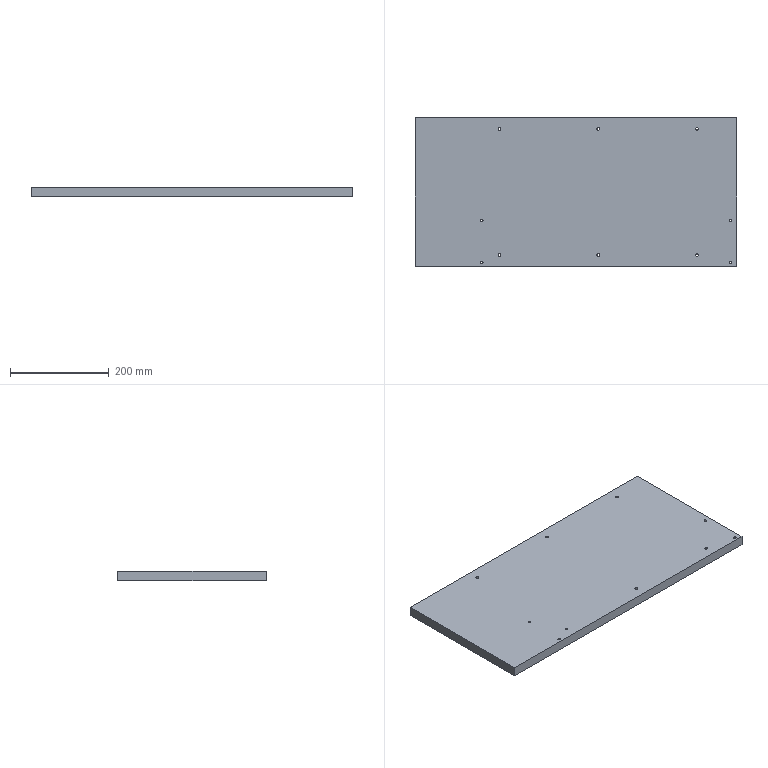Part | SolidWorks | features BaseBody 1 | 1 solid | 44 faces | box 650 x 300 x 20 mm | volume 3893705 mm3 | cylinder 32 | plane 12 | commonest cylinder face diameters 5.5 x12 10 x12 5 x8
STEP:
#1=CARTESIAN_POINT('',(240.,-127.5,5.7));
#2=VERTEX_POINT('',#1);
#3=CARTESIAN_POINT('',(250.,-127.5,5.7));
#4=VERTEX_POINT('',#3);
#5=CARTESIAN_POINT('',(245.,-127.5,5.7));
#6=DIRECTION('',(0.,0.,1.));
#7=DIRECTION('',(-1.,0.,0.));
#8=AXIS2_PLACEMENT_3D('',#5,#6,#7);
#9=CIRCLE('',#8,5.);
#10=EDGE_CURVE('',#2,#4,#9,.T.);
#11=ORIENTED_EDGE('',*,*,#10,.T.);
#12=CARTESIAN_POINT('',(250.,-127.5,0.));
#13=VERTEX_POINT('',#12);
#14=CARTESIAN_POINT('',(250.,-127.5,5.7));
#15=DIRECTION('',(0.,0.,-1.));
#16=VECTOR('',#15,1000.);
#17=LINE('',#14,#16);
#18=EDGE_CURVE('',#4,#13,#17,.T.);
#19=ORIENTED_EDGE('',*,*,#18,.T.);
#20=CARTESIAN_POINT('',(240.,-127.5,0.));
#21=VERTEX_POINT('',#20);
#22=CARTESIAN_POINT('',(245.,-127.5,0.));
#23=DIRECTION('',(0.,0.,-1.));
#24=DIRECTION('',(-1.,0.,0.));
#25=AXIS2_PLACEMENT_3D('',#22,#23,#24);
#26=CIRCLE('',#25,5.);
#27=EDGE_CURVE('',#13,#21,#26,.T.);
#28=ORIENTED_EDGE('',*,*,#27,.T.);
#29=CARTESIAN_POINT('',(240.,-127.5,5.7));
#30=DIRECTION('',(0.,0.,-1.));
#31=VECTOR('',#30,1000.);
#32=LINE('',#29,#31);
#33=EDGE_CURVE('',#2,#21,#32,.T.);
#34=ORIENTED_EDGE('',*,*,#33,.F.);
#35=EDGE_LOOP('',(#11,#19,#28,#34));
#36=FACE_OUTER_BOUND('',#35,.T.);
#37=CARTESIAN_POINT('',(245.,-127.5,5.7));
#38=DIRECTION('',(0.,0.,-1.));
#39=DIRECTION('',(-1.,0.,0.));
#40=AXIS2_PLACEMENT_3D('',#37,#38,#39);
#41=CYLINDRICAL_SURFACE('',#40,5.);
#42=ADVANCED_FACE('',(#36),#41,.F.);
#43=CARTESIAN_POINT('',(315.,-57.5,0.));
#44=VERTEX_POINT('',#43);
#45=CARTESIAN_POINT('',(310.,-57.5,0.));
#46=VERTEX_POINT('',#45);
#47=CARTESIAN_POINT('',(312.5,-57.5,0.));
#48=DIRECTION('',(0.,0.,-1.));
#49=DIRECTION('',(1.,0.,0.));
#50=AXIS2_PLACEMENT_3D('',#47,#48,#49);
#51=CIRCLE('',#50,2.5);
#52=EDGE_CURVE('',#44,#46,#51,.T.);
#53=ORIENTED_EDGE('',*,*,#52,.T.);
#54=CARTESIAN_POINT('',(310.,-57.5,20.));
#55=VERTEX_POINT('',#54);
#56=CARTESIAN_POINT('',(310.,-57.5,0.));
#57=DIRECTION('',(0.,0.,1.));
#58=VECTOR('',#57,1000.);
#59=LINE('',#56,#58);
#60=EDGE_CURVE('',#46,#55,#59,.T.);
#61=ORIENTED_EDGE('',*,*,#60,.T.);
#62=CARTESIAN_POINT('',(315.,-57.5,20.));
#63=VERTEX_POINT('',#62);
#64=CARTESIAN_POINT('',(312.5,-57.5,20.));
#65=DIRECTION('',(0.,0.,1.));
#66=DIRECTION('',(1.,0.,0.));
#67=AXIS2_PLACEMENT_3D('',#64,#65,#66);
#68=CIRCLE('',#67,2.5);
#69=EDGE_CURVE('',#55,#63,#68,.T.);
#70=ORIENTED_EDGE('',*,*,#69,.T.);
#71=CARTESIAN_POINT('',(315.,-57.5,0.));
#72=DIRECTION('',(0.,0.,1.));
#73=VECTOR('',#72,1000.);
#74=LINE('',#71,#73);
#75=EDGE_CURVE('',#44,#63,#74,.T.);
#76=ORIENTED_EDGE('',*,*,#75,.F.);
#77=EDGE_LOOP('',(#53,#61,#70,#76));
#78=FACE_OUTER_BOUND('',#77,.T.);
#79=CARTESIAN_POINT('',(312.5,-57.5,0.));
#80=DIRECTION('',(0.,0.,1.));
#81=DIRECTION('',(1.,0.,0.));
#82=AXIS2_PLACEMENT_3D('',#79,#80,#81);
#83=CYLINDRICAL_SURFACE('',#82,2.5);
#84=ADVANCED_FACE('',(#78),#83,.F.);
#85=CARTESIAN_POINT('',(-188.,-142.5,0.));
#86=VERTEX_POINT('',#85);
#87=CARTESIAN_POINT('',(-193.,-142.5,0.));
#88=VERTEX_POINT('',#87);
#89=CARTESIAN_POINT('',(-190.5,-142.5,0.));
#90=DIRECTION('',(0.,0.,-1.));
#91=DIRECTION('',(1.,0.,0.));
#92=AXIS2_PLACEMENT_3D('',#89,#90,#91);
#93=CIRCLE('',#92,2.5);
#94=EDGE_CURVE('',#86,#88,#93,.T.);
#95=ORIENTED_EDGE('',*,*,#94,.T.);
#96=CARTESIAN_POINT('',(-193.,-142.5,20.));
#97=VERTEX_POINT('',#96);
#98=CARTESIAN_POINT('',(-193.,-142.5,0.));
#99=DIRECTION('',(0.,0.,1.));
#100=VECTOR('',#99,1000.);
#101=LINE('',#98,#100);
#102=EDGE_CURVE('',#88,#97,#101,.T.);
#103=ORIENTED_EDGE('',*,*,#102,.T.);
#104=CARTESIAN_POINT('',(-188.,-142.5,20.));
#105=VERTEX_POINT('',#104);
#106=CARTESIAN_POINT('',(-190.5,-142.5,20.));
#107=DIRECTION('',(0.,0.,1.));
#108=DIRECTION('',(1.,0.,0.));
#109=AXIS2_PLACEMENT_3D('',#106,#107,#108);
#110=CIRCLE('',#109,2.5);
#111=EDGE_CURVE('',#97,#105,#110,.T.);
#112=ORIENTED_EDGE('',*,*,#111,.T.);
#113=CARTESIAN_POINT('',(-188.,-142.5,0.));
#114=DIRECTION('',(0.,0.,1.));
#115=VECTOR('',#114,1000.);
#116=LINE('',#113,#115);
#117=EDGE_CURVE('',#86,#105,#116,.T.);
#118=ORIENTED_EDGE('',*,*,#117,.F.);
#119=EDGE_LOOP('',(#95,#103,#112,#118));
#120=FACE_OUTER_BOUND('',#119,.T.);
#121=CARTESIAN_POINT('',(-190.5,-142.5,0.));
#122=DIRECTION('',(0.,0.,1.));
#123=DIRECTION('',(1.,0.,0.));
#124=AXIS2_PLACEMENT_3D('',#121,#122,#123);
#125=CYLINDRICAL_SURFACE('',#124,2.5);
#126=ADVANCED_FACE('',(#120),#125,.F.);
#127=CARTESIAN_POINT('',(-188.,-57.5,0.));
#128=VERTEX_POINT('',#127);
#129=CARTESIAN_POINT('',(-193.,-57.5,0.));
#130=VERTEX_POINT('',#129);
#131=CARTESIAN_POINT('',(-190.5,-57.5,0.));
#132=DIRECTION('',(0.,0.,-1.));
#133=DIRECTION('',(1.,0.,0.));
#134=AXIS2_PLACEMENT_3D('',#131,#132,#133);
#135=CIRCLE('',#134,2.5);
#136=EDGE_CURVE('',#128,#130,#135,.T.);
#137=ORIENTED_EDGE('',*,*,#136,.T.);
#138=CARTESIAN_POINT('',(-193.,-57.5,20.));
#139=VERTEX_POINT('',#138);
#140=CARTESIAN_POINT('',(-193.,-57.5,0.));
#141=DIRECTION('',(0.,0.,1.));
#142=VECTOR('',#141,1000.);
#143=LINE('',#140,#142);
#144=EDGE_CURVE('',#130,#139,#143,.T.);
#145=ORIENTED_EDGE('',*,*,#144,.T.);
#146=CARTESIAN_POINT('',(-188.,-57.5,20.));
#147=VERTEX_POINT('',#146);
#148=CARTESIAN_POINT('',(-190.5,-57.5,20.));
#149=DIRECTION('',(0.,0.,1.));
#150=DIRECTION('',(1.,0.,0.));
#151=AXIS2_PLACEMENT_3D('',#148,#149,#150);
#152=CIRCLE('',#151,2.5);
#153=EDGE_CURVE('',#139,#147,#152,.T.);
#154=ORIENTED_EDGE('',*,*,#153,.T.);
#155=CARTESIAN_POINT('',(-188.,-57.5,0.));
#156=DIRECTION('',(0.,0.,1.));
#157=VECTOR('',#156,1000.);
#158=LINE('',#155,#157);
#159=EDGE_CURVE('',#128,#147,#158,.T.);
#160=ORIENTED_EDGE('',*,*,#159,.F.);
#161=EDGE_LOOP('',(#137,#145,#154,#160));
#162=FACE_OUTER_BOUND('',#161,.T.);
#163=CARTESIAN_POINT('',(-190.5,-57.5,0.));
#164=DIRECTION('',(0.,0.,1.));
#165=DIRECTION('',(1.,0.,0.));
#166=AXIS2_PLACEMENT_3D('',#163,#164,#165);
#167=CYLINDRICAL_SURFACE('',#166,2.5);
#168=ADVANCED_FACE('',(#162),#167,.F.);
#169=CARTESIAN_POINT('',(315.,-142.5,0.));
#170=VERTEX_POINT('',#169);
#171=CARTESIAN_POINT('',(310.,-142.5,0.));
#172=VERTEX_POINT('',#171);
#173=CARTESIAN_POINT('',(312.5,-142.5,0.));
#174=DIRECTION('',(0.,0.,-1.));
#175=DIRECTION('',(1.,0.,0.));
#176=AXIS2_PLACEMENT_3D('',#173,#174,#175);
#177=CIRCLE('',#176,2.5);
#178=EDGE_CURVE('',#170,#172,#177,.T.);
#179=ORIENTED_EDGE('',*,*,#178,.T.);
#180=CARTESIAN_POINT('',(310.,-142.5,20.));
#181=VERTEX_POINT('',#180);
#182=CARTESIAN_POINT('',(310.,-142.5,0.));
#183=DIRECTION('',(0.,0.,1.));
#184=VECTOR('',#183,1000.);
#185=LINE('',#182,#184);
#186=EDGE_CURVE('',#172,#181,#185,.T.);
#187=ORIENTED_EDGE('',*,*,#186,.T.);
#188=CARTESIAN_POINT('',(315.,-142.5,20.));
#189=VERTEX_POINT('',#188);
#190=CARTESIAN_POINT('',(312.5,-142.5,20.));
#191=DIRECTION('',(0.,0.,1.));
#192=DIRECTION('',(1.,0.,0.));
#193=AXIS2_PLACEMENT_3D('',#190,#191,#192);
#194=CIRCLE('',#193,2.5);
#195=EDGE_CURVE('',#181,#189,#194,.T.);
#196=ORIENTED_EDGE('',*,*,#195,.T.);
#197=CARTESIAN_POINT('',(315.,-142.5,0.));
#198=DIRECTION('',(0.,0.,1.));
#199=VECTOR('',#198,1000.);
#200=LINE('',#197,#199);
#201=EDGE_CURVE('',#170,#189,#200,.T.);
#202=ORIENTED_EDGE('',*,*,#201,.F.);
#203=EDGE_LOOP('',(#179,#187,#196,#202));
#204=FACE_OUTER_BOUND('',#203,.T.);
#205=CARTESIAN_POINT('',(312.5,-142.5,0.));
#206=DIRECTION('',(0.,0.,1.));
#207=DIRECTION('',(1.,0.,0.));
#208=AXIS2_PLACEMENT_3D('',#205,#206,#207);
#209=CYLINDRICAL_SURFACE('',#208,2.5);
#210=ADVANCED_FACE('',(#204),#209,.F.);
#211=CARTESIAN_POINT('',(240.,127.5,5.7));
#212=VERTEX_POINT('',#211);
#213=CARTESIAN_POINT('',(250.,127.5,5.7));
#214=VERTEX_POINT('',#213);
#215=CARTESIAN_POINT('',(245.,127.5,5.7));
#216=DIRECTION('',(0.,0.,1.));
#217=DIRECTION('',(-1.,0.,0.));
#218=AXIS2_PLACEMENT_3D('',#215,#216,#217);
#219=CIRCLE('',#218,5.);
#220=EDGE_CURVE('',#212,#214,#219,.T.);
#221=ORIENTED_EDGE('',*,*,#220,.T.);
#222=CARTESIAN_POINT('',(250.,127.5,0.));
#223=VERTEX_POINT('',#222);
#224=CARTESIAN_POINT('',(250.,127.5,5.7));
#225=DIRECTION('',(0.,0.,-1.));
#226=VECTOR('',#225,1000.);
#227=LINE('',#224,#226);
#228=EDGE_CURVE('',#214,#223,#227,.T.);
#229=ORIENTED_EDGE('',*,*,#228,.T.);
#230=CARTESIAN_POINT('',(240.,127.5,0.));
#231=VERTEX_POINT('',#230);
#232=CARTESIAN_POINT('',(245.,127.5,0.));
#233=DIRECTION('',(0.,0.,-1.));
#234=DIRECTION('',(-1.,0.,0.));
#235=AXIS2_PLACEMENT_3D('',#232,#233,#234);
#236=CIRCLE('',#235,5.);
#237=EDGE_CURVE('',#223,#231,#236,.T.);
#238=ORIENTED_EDGE('',*,*,#237,.T.);
#239=CARTESIAN_POINT('',(240.,127.5,5.7));
#240=DIRECTION('',(0.,0.,-1.));
#241=VECTOR('',#240,1000.);
#242=LINE('',#239,#241);
#243=EDGE_CURVE('',#212,#231,#242,.T.);
#244=ORIENTED_EDGE('',*,*,#243,.F.);
#245=EDGE_LOOP('',(#221,#229,#238,#244));
#246=FACE_OUTER_BOUND('',#245,.T.);
#247=CARTESIAN_POINT('',(245.,127.5,5.7));
#248=DIRECTION('',(0.,0.,-1.));
#249=DIRECTION('',(-1.,0.,0.));
#250=AXIS2_PLACEMENT_3D('',#247,#248,#249);
#251=CYLINDRICAL_SURFACE('',#250,5.);
#252=ADVANCED_FACE('',(#246),#251,.F.);
#253=CARTESIAN_POINT('',(40.,127.5,5.7));
#254=VERTEX_POINT('',#253);
#255=CARTESIAN_POINT('',(50.,127.5,5.7));
#256=VERTEX_POINT('',#255);
#257=CARTESIAN_POINT('',(45.,127.5,5.7));
#258=DIRECTION('',(0.,0.,1.));
#259=DIRECTION('',(-1.,0.,0.));
#260=AXIS2_PLACEMENT_3D('',#257,#258,#259);
#261=CIRCLE('',#260,5.);
#262=EDGE_CURVE('',#254,#256,#261,.T.);
#263=ORIENTED_EDGE('',*,*,#262,.T.);
#264=CARTESIAN_POINT('',(50.,127.5,0.));
#265=VERTEX_POINT('',#264);
#266=CARTESIAN_POINT('',(50.,127.5,5.7));
#267=DIRECTION('',(0.,0.,-1.));
#268=VECTOR('',#267,1000.);
#269=LINE('',#266,#268);
#270=EDGE_CURVE('',#256,#265,#269,.T.);
#271=ORIENTED_EDGE('',*,*,#270,.T.);
#272=CARTESIAN_POINT('',(40.,127.5,0.));
#273=VERTEX_POINT('',#272);
#274=CARTESIAN_POINT('',(45.,127.5,0.));
#275=DIRECTION('',(0.,0.,-1.));
#276=DIRECTION('',(-1.,0.,0.));
#277=AXIS2_PLACEMENT_3D('',#274,#275,#276);
#278=CIRCLE('',#277,5.);
#279=EDGE_CURVE('',#265,#273,#278,.T.);
#280=ORIENTED_EDGE('',*,*,#279,.T.);
#281=CARTESIAN_POINT('',(40.,127.5,5.7));
#282=DIRECTION('',(0.,0.,-1.));
#283=VECTOR('',#282,1000.);
#284=LINE('',#281,#283);
#285=EDGE_CURVE('',#254,#273,#284,.T.);
#286=ORIENTED_EDGE('',*,*,#285,.F.);
#287=EDGE_LOOP('',(#263,#271,#280,#286));
#288=FACE_OUTER_BOUND('',#287,.T.);
#289=CARTESIAN_POINT('',(45.,127.5,5.7));
#290=DIRECTION('',(0.,0.,-1.));
#291=DIRECTION('',(-1.,0.,0.));
#292=AXIS2_PLACEMENT_3D('',#289,#290,#291);
#293=CYLINDRICAL_SURFACE('',#292,5.);
#294=ADVANCED_FACE('',(#288),#293,.F.);
#295=CARTESIAN_POINT('',(-160.,127.5,5.7));
#296=VERTEX_POINT('',#295);
#297=CARTESIAN_POINT('',(-150.,127.5,5.7));
#298=VERTEX_POINT('',#297);
#299=CARTESIAN_POINT('',(-155.,127.5,5.7));
#300=DIRECTION('',(0.,0.,1.));
#301=DIRECTION('',(-1.,0.,0.));
#302=AXIS2_PLACEMENT_3D('',#299,#300,#301);
#303=CIRCLE('',#302,5.);
#304=EDGE_CURVE('',#296,#298,#303,.T.);
#305=ORIENTED_EDGE('',*,*,#304,.T.);
#306=CARTESIAN_POINT('',(-150.,127.5,0.));
#307=VERTEX_POINT('',#306);
#308=CARTESIAN_POINT('',(-150.,127.5,5.7));
#309=DIRECTION('',(0.,0.,-1.));
#310=VECTOR('',#309,1000.);
#311=LINE('',#308,#310);
#312=EDGE_CURVE('',#298,#307,#311,.T.);
#313=ORIENTED_EDGE('',*,*,#312,.T.);
#314=CARTESIAN_POINT('',(-160.,127.5,0.));
#315=VERTEX_POINT('',#314);
#316=CARTESIAN_POINT('',(-155.,127.5,0.));
#317=DIRECTION('',(0.,0.,-1.));
#318=DIRECTION('',(-1.,0.,0.));
#319=AXIS2_PLACEMENT_3D('',#316,#317,#318);
#320=CIRCLE('',#319,5.);
#321=EDGE_CURVE('',#307,#315,#320,.T.);
#322=ORIENTED_EDGE('',*,*,#321,.T.);
#323=CARTESIAN_POINT('',(-160.,127.5,5.7));
#324=DIRECTION('',(0.,0.,-1.));
#325=VECTOR('',#324,1000.);
#326=LINE('',#323,#325);
#327=EDGE_CURVE('',#296,#315,#326,.T.);
#328=ORIENTED_EDGE('',*,*,#327,.F.);
#329=EDGE_LOOP('',(#305,#313,#322,#328));
#330=FACE_OUTER_BOUND('',#329,.T.);
#331=CARTESIAN_POINT('',(-155.,127.5,5.7));
#332=DIRECTION('',(0.,0.,-1.));
#333=DIRECTION('',(-1.,0.,0.));
#334=AXIS2_PLACEMENT_3D('',#331,#332,#333);
#335=CYLINDRICAL_SURFACE('',#334,5.);
#336=ADVANCED_FACE('',(#330),#335,.F.);
#337=CARTESIAN_POINT('',(-160.,-127.5,5.7));
#338=VERTEX_POINT('',#337);
#339=CARTESIAN_POINT('',(-150.,-127.5,5.7));
#340=VERTEX_POINT('',#339);
#341=CARTESIAN_POINT('',(-155.,-127.5,5.7));
#342=DIRECTION('',(0.,0.,1.));
#343=DIRECTION('',(-1.,0.,0.));
#344=AXIS2_PLACEMENT_3D('',#341,#342,#343);
#345=CIRCLE('',#344,5.);
#346=EDGE_CURVE('',#338,#340,#345,.T.);
#347=ORIENTED_EDGE('',*,*,#346,.T.);
#348=CARTESIAN_POINT('',(-150.,-127.5,0.));
#349=VERTEX_POINT('',#348);
#350=CARTESIAN_POINT('',(-150.,-127.5,5.7));
#351=DIRECTION('',(0.,0.,-1.));
#352=VECTOR('',#351,1000.);
#353=LINE('',#350,#352);
#354=EDGE_CURVE('',#340,#349,#353,.T.);
#355=ORIENTED_EDGE('',*,*,#354,.T.);
#356=CARTESIAN_POINT('',(-160.,-127.5,0.));
#357=VERTEX_POINT('',#356);
#358=CARTESIAN_POINT('',(-155.,-127.5,0.));
#359=DIRECTION('',(0.,0.,-1.));
#360=DIRECTION('',(-1.,0.,0.));
#361=AXIS2_PLACEMENT_3D('',#358,#359,#360);
#362=CIRCLE('',#361,5.);
#363=EDGE_CURVE('',#349,#357,#362,.T.);
#364=ORIENTED_EDGE('',*,*,#363,.T.);
#365=CARTESIAN_POINT('',(-160.,-127.5,5.7));
#366=DIRECTION('',(0.,0.,-1.));
#367=VECTOR('',#366,1000.);
#368=LINE('',#365,#367);
#369=EDGE_CURVE('',#338,#357,#368,.T.);
#370=ORIENTED_EDGE('',*,*,#369,.F.);
#371=EDGE_LOOP('',(#347,#355,#364,#370));
#372=FACE_OUTER_BOUND('',#371,.T.);
#373=CARTESIAN_POINT('',(-155.,-127.5,5.7));
#374=DIRECTION('',(0.,0.,-1.));
#375=DIRECTION('',(-1.,0.,0.));
#376=AXIS2_PLACEMENT_3D('',#373,#374,#375);
#377=CYLINDRICAL_SURFACE('',#376,5.);
#378=ADVANCED_FACE('',(#372),#377,.F.);
#379=CARTESIAN_POINT('',(40.,-127.5,5.7));
#380=VERTEX_POINT('',#379);
#381=CARTESIAN_POINT('',(50.,-127.5,5.7));
#382=VERTEX_POINT('',#381);
#383=CARTESIAN_POINT('',(45.,-127.5,5.7));
#384=DIRECTION('',(0.,0.,1.));
#385=DIRECTION('',(-1.,0.,0.));
#386=AXIS2_PLACEMENT_3D('',#383,#384,#385);
#387=CIRCLE('',#386,5.);
#388=EDGE_CURVE('',#380,#382,#387,.T.);
#389=ORIENTED_EDGE('',*,*,#388,.T.);
#390=CARTESIAN_POINT('',(50.,-127.5,0.));
#391=VERTEX_POINT('',#390);
#392=CARTESIAN_POINT('',(50.,-127.5,5.7));
#393=DIRECTION('',(0.,0.,-1.));
#394=VECTOR('',#393,1000.);
#395=LINE('',#392,#394);
#396=EDGE_CURVE('',#382,#391,#395,.T.);
#397=ORIENTED_EDGE('',*,*,#396,.T.);
#398=CARTESIAN_POINT('',(40.,-127.5,0.));
#399=VERTEX_POINT('',#398);
#400=CARTESIAN_POINT('',(45.,-127.5,0.));
#401=DIRECTION('',(0.,0.,-1.));
#402=DIRECTION('',(-1.,0.,0.));
#403=AXIS2_PLACEMENT_3D('',#400,#401,#402);
#404=CIRCLE('',#403,5.);
#405=EDGE_CURVE('',#391,#399,#404,.T.);
#406=ORIENTED_EDGE('',*,*,#405,.T.);
#407=CARTESIAN_POINT('',(40.,-127.5,5.7));
#408=DIRECTION('',(0.,0.,-1.));
#409=VECTOR('',#408,1000.);
#410=LINE('',#407,#409);
#411=EDGE_CURVE('',#380,#399,#410,.T.);
#412=ORIENTED_EDGE('',*,*,#411,.F.);
#413=EDGE_LOOP('',(#389,#397,#406,#412));
#414=FACE_OUTER_BOUND('',#413,.T.);
#415=CARTESIAN_POINT('',(45.,-127.5,5.7));
#416=DIRECTION('',(0.,0.,-1.));
#417=DIRECTION('',(-1.,0.,0.));
#418=AXIS2_PLACEMENT_3D('',#415,#416,#417);
#419=CYLINDRICAL_SURFACE('',#418,5.);
#420=ADVANCED_FACE('',(#414),#419,.F.);
#421=CARTESIAN_POINT('',(245.,-124.75,20.));
#422=VERTEX_POINT('',#421);
#423=CARTESIAN_POINT('',(245.,-130.25,20.));
#424=VERTEX_POINT('',#423);
#425=CARTESIAN_POINT('',(245.,-127.5,20.));
#426=DIRECTION('',(0.,0.,1.));
#427=DIRECTION('',(0.,1.,0.));
#428=AXIS2_PLACEMENT_3D('',#425,#426,#427);
#429=CIRCLE('',#428,2.75);
#430=EDGE_CURVE('',#422,#424,#429,.T.);
#431=ORIENTED_EDGE('',*,*,#430,.T.);
#432=CARTESIAN_POINT('',(245.,-130.25,5.7));
#433=VERTEX_POINT('',#432);
#434=CARTESIAN_POINT('',(245.,-130.25,20.));
#435=DIRECTION('',(0.,0.,-1.));
#436=VECTOR('',#435,1000.);
#437=LINE('',#434,#436);
#438=EDGE_CURVE('',#424,#433,#437,.T.);
#439=ORIENTED_EDGE('',*,*,#438,.T.);
#440=CARTESIAN_POINT('',(245.,-124.75,5.7));
#441=VERTEX_POINT('',#440);
#442=CARTESIAN_POINT('',(245.,-127.5,5.7));
#443=DIRECTION('',(0.,0.,-1.));
#444=DIRECTION('',(0.,1.,0.));
#445=AXIS2_PLACEMENT_3D('',#442,#443,#444);
#446=CIRCLE('',#445,2.75);
#447=EDGE_CURVE('',#433,#441,#446,.T.);
#448=ORIENTED_EDGE('',*,*,#447,.T.);
#449=CARTESIAN_POINT('',(245.,-124.75,20.));
#450=DIRECTION('',(0.,0.,-1.));
#451=VECTOR('',#450,1000.);
#452=LINE('',#449,#451);
#453=EDGE_CURVE('',#422,#441,#452,.T.);
#454=ORIENTED_EDGE('',*,*,#453,.F.);
#455=EDGE_LOOP('',(#431,#439,#448,#454));
#456=FACE_OUTER_BOUND('',#455,.T.);
#457=CARTESIAN_POINT('',(245.,-127.5,20.));
#458=DIRECTION('',(0.,0.,-1.));
#459=DIRECTION('',(0.,1.,0.));
#460=AXIS2_PLACEMENT_3D('',#457,#458,#459);
#461=CYLINDRICAL_SURFACE('',#460,2.75);
#462=ADVANCED_FACE('',(#456),#461,.F.);
#463=CARTESIAN_POINT('',(245.,124.75,20.));
#464=VERTEX_POINT('',#463);
#465=CARTESIAN_POINT('',(245.,130.25,20.));
#466=VERTEX_POINT('',#465);
#467=CARTESIAN_POINT('',(245.,127.5,20.));
#468=DIRECTION('',(0.,0.,-1.));
#469=DIRECTION('',(0.,1.,0.));
#470=AXIS2_PLACEMENT_3D('',#467,#468,#469);
#471=CIRCLE('',#470,2.75);
#472=EDGE_CURVE('',#464,#466,#471,.T.);
#473=ORIENTED_EDGE('',*,*,#472,.F.);
#474=CARTESIAN_POINT('',(245.,124.75,5.7));
#475=VERTEX_POINT('',#474);
#476=CARTESIAN_POINT('',(245.,124.75,20.));
#477=DIRECTION('',(0.,0.,-1.));
#478=VECTOR('',#477,1000.);
#479=LINE('',#476,#478);
#480=EDGE_CURVE('',#464,#475,#479,.T.);
#481=ORIENTED_EDGE('',*,*,#480,.T.);
#482=CARTESIAN_POINT('',(245.,130.25,5.7));
#483=VERTEX_POINT('',#482);
#484=CARTESIAN_POINT('',(245.,127.5,5.7));
#485=DIRECTION('',(0.,0.,-1.));
#486=DIRECTION('',(0.,1.,0.));
#487=AXIS2_PLACEMENT_3D('',#484,#485,#486);
#488=CIRCLE('',#487,2.75);
#489=EDGE_CURVE('',#475,#483,#488,.T.);
#490=ORIENTED_EDGE('',*,*,#489,.T.);
#491=CARTESIAN_POINT('',(245.,130.25,20.));
#492=DIRECTION('',(0.,0.,-1.));
#493=VECTOR('',#492,1000.);
#494=LINE('',#491,#493);
#495=EDGE_CURVE('',#466,#483,#494,.T.);
#496=ORIENTED_EDGE('',*,*,#495,.F.);
#497=EDGE_LOOP('',(#473,#481,#490,#496));
#498=FACE_OUTER_BOUND('',#497,.T.);
#499=CARTESIAN_POINT('',(245.,127.5,20.));
#500=DIRECTION('',(0.,0.,-1.));
#501=DIRECTION('',(0.,1.,0.));
#502=AXIS2_PLACEMENT_3D('',#499,#500,#501);
#503=CYLINDRICAL_SURFACE('',#502,2.75);
#504=ADVANCED_FACE('',(#498),#503,.F.);
#505=CARTESIAN_POINT('',(45.,124.75,20.));
#506=VERTEX_POINT('',#505);
#507=CARTESIAN_POINT('',(45.,130.25,20.));
#508=VERTEX_POINT('',#507);
#509=CARTESIAN_POINT('',(45.,127.5,20.));
#510=DIRECTION('',(0.,0.,-1.));
#511=DIRECTION('',(0.,1.,0.));
#512=AXIS2_PLACEMENT_3D('',#509,#510,#511);
#513=CIRCLE('',#512,2.75);
#514=EDGE_CURVE('',#506,#508,#513,.T.);
#515=ORIENTED_EDGE('',*,*,#514,.F.);
#516=CARTESIAN_POINT('',(45.,124.75,5.7));
#517=VERTEX_POINT('',#516);
#518=CARTESIAN_POINT('',(45.,124.75,20.));
#519=DIRECTION('',(0.,0.,-1.));
#520=VECTOR('',#519,1000.);
#521=LINE('',#518,#520);
#522=EDGE_CURVE('',#506,#517,#521,.T.);
#523=ORIENTED_EDGE('',*,*,#522,.T.);
#524=CARTESIAN_POINT('',(45.,130.25,5.7));
#525=VERTEX_POINT('',#524);
#526=CARTESIAN_POINT('',(45.,127.5,5.7));
#527=DIRECTION('',(0.,0.,-1.));
#528=DIRECTION('',(0.,1.,0.));
#529=AXIS2_PLACEMENT_3D('',#526,#527,#528);
#530=CIRCLE('',#529,2.75);
#531=EDGE_CURVE('',#517,#525,#530,.T.);
#532=ORIENTED_EDGE('',*,*,#531,.T.);
#533=CARTESIAN_POINT('',(45.,130.25,20.));
#534=DIRECTION('',(0.,0.,-1.));
#535=VECTOR('',#534,1000.);
#536=LINE('',#533,#535);
#537=EDGE_CURVE('',#508,#525,#536,.T.);
#538=ORIENTED_EDGE('',*,*,#537,.F.);
#539=EDGE_LOOP('',(#515,#523,#532,#538));
#540=FACE_OUTER_BOUND('',#539,.T.);
#541=CARTESIAN_POINT('',(45.,127.5,20.));
#542=DIRECTION('',(0.,0.,-1.));
#543=DIRECTION('',(0.,1.,0.));
#544=AXIS2_PLACEMENT_3D('',#541,#542,#543);
#545=CYLINDRICAL_SURFACE('',#544,2.75);
#546=ADVANCED_FACE('',(#540),#545,.F.);
#547=CARTESIAN_POINT('',(-155.,124.75,20.));
#548=VERTEX_POINT('',#547);
#549=CARTESIAN_POINT('',(-155.,130.25,20.));
#550=VERTEX_POINT('',#549);
#551=CARTESIAN_POINT('',(-155.,127.5,20.));
#552=DIRECTION('',(0.,0.,-1.));
#553=DIRECTION('',(0.,1.,0.));
#554=AXIS2_PLACEMENT_3D('',#551,#552,#553);
#555=CIRCLE('',#554,2.75);
#556=EDGE_CURVE('',#548,#550,#555,.T.);
#557=ORIENTED_EDGE('',*,*,#556,.F.);
#558=CARTESIAN_POINT('',(-155.,124.75,5.7));
#559=VERTEX_POINT('',#558);
#560=CARTESIAN_POINT('',(-155.,124.75,20.));
#561=DIRECTION('',(0.,0.,-1.));
#562=VECTOR('',#561,1000.);
#563=LINE('',#560,#562);
#564=EDGE_CURVE('',#548,#559,#563,.T.);
#565=ORIENTED_EDGE('',*,*,#564,.T.);
#566=CARTESIAN_POINT('',(-155.,130.25,5.7));
#567=VERTEX_POINT('',#566);
#568=CARTESIAN_POINT('',(-155.,127.5,5.7));
#569=DIRECTION('',(0.,0.,-1.));
#570=DIRECTION('',(0.,1.,0.));
#571=AXIS2_PLACEMENT_3D('',#568,#569,#570);
#572=CIRCLE('',#571,2.75);
#573=EDGE_CURVE('',#559,#567,#572,.T.);
#574=ORIENTED_EDGE('',*,*,#573,.T.);
#575=CARTESIAN_POINT('',(-155.,130.25,20.));
#576=DIRECTION('',(0.,0.,-1.));
#577=VECTOR('',#576,1000.);
#578=LINE('',#575,#577);
#579=EDGE_CURVE('',#550,#567,#578,.T.);
#580=ORIENTED_EDGE('',*,*,#579,.F.);
#581=EDGE_LOOP('',(#557,#565,#574,#580));
#582=FACE_OUTER_BOUND('',#581,.T.);
#583=CARTESIAN_POINT('',(-155.,127.5,20.));
#584=DIRECTION('',(0.,0.,-1.));
#585=DIRECTION('',(0.,1.,0.));
#586=AXIS2_PLACEMENT_3D('',#583,#584,#585);
#587=CYLINDRICAL_SURFACE('',#586,2.75);
#588=ADVANCED_FACE('',(#582),#587,.F.);
#589=CARTESIAN_POINT('',(-155.,-130.25,20.));
#590=VERTEX_POINT('',#589);
#591=CARTESIAN_POINT('',(-155.,-124.75,20.));
#592=VERTEX_POINT('',#591);
#593=CARTESIAN_POINT('',(-155.,-127.5,20.));
#594=DIRECTION('',(0.,0.,-1.));
#595=DIRECTION('',(0.,1.,0.));
#596=AXIS2_PLACEMENT_3D('',#593,#594,#595);
#597=CIRCLE('',#596,2.75);
#598=EDGE_CURVE('',#590,#592,#597,.T.);
#599=ORIENTED_EDGE('',*,*,#598,.F.);
#600=CARTESIAN_POINT('',(-155.,-130.25,5.7));
#601=VERTEX_POINT('',#600);
#602=CARTESIAN_POINT('',(-155.,-130.25,20.));
#603=DIRECTION('',(0.,0.,-1.));
#604=VECTOR('',#603,1000.);
#605=LINE('',#602,#604);
#606=EDGE_CURVE('',#590,#601,#605,.T.);
#607=ORIENTED_EDGE('',*,*,#606,.T.);
#608=CARTESIAN_POINT('',(-155.,-124.75,5.7));
#609=VERTEX_POINT('',#608);
#610=CARTESIAN_POINT('',(-155.,-127.5,5.7));
#611=DIRECTION('',(0.,0.,-1.));
#612=DIRECTION('',(0.,1.,0.));
#613=AXIS2_PLACEMENT_3D('',#610,#611,#612);
#614=CIRCLE('',#613,2.75);
#615=EDGE_CURVE('',#601,#609,#614,.T.);
#616=ORIENTED_EDGE('',*,*,#615,.T.);
#617=CARTESIAN_POINT('',(-155.,-124.75,20.));
#618=DIRECTION('',(0.,0.,-1.));
#619=VECTOR('',#618,1000.);
#620=LINE('',#617,#619);
#621=EDGE_CURVE('',#592,#609,#620,.T.);
#622=ORIENTED_EDGE('',*,*,#621,.F.);
#623=EDGE_LOOP('',(#599,#607,#616,#622));
#624=FACE_OUTER_BOUND('',#623,.T.);
#625=CARTESIAN_POINT('',(-155.,-127.5,20.));
#626=DIRECTION('',(0.,0.,-1.));
#627=DIRECTION('',(0.,1.,0.));
#628=AXIS2_PLACEMENT_3D('',#625,#626,#627);
#629=CYLINDRICAL_SURFACE('',#628,2.75);
#630=ADVANCED_FACE('',(#624),#629,.F.);
#631=CARTESIAN_POINT('',(45.,-130.25,20.));
#632=VERTEX_POINT('',#631);
#633=CARTESIAN_POINT('',(45.,-124.75,20.));
#634=VERTEX_POINT('',#633);
#635=CARTESIAN_POINT('',(45.,-127.5,20.));
#636=DIRECTION('',(0.,0.,-1.));
#637=DIRECTION('',(0.,1.,0.));
#638=AXIS2_PLACEMENT_3D('',#635,#636,#637);
#639=CIRCLE('',#638,2.75);
#640=EDGE_CURVE('',#632,#634,#639,.T.);
#641=ORIENTED_EDGE('',*,*,#640,.F.);
#642=CARTESIAN_POINT('',(45.,-130.25,5.7));
#643=VERTEX_POINT('',#642);
#644=CARTESIAN_POINT('',(45.,-130.25,20.));
#645=DIRECTION('',(0.,0.,-1.));
#646=VECTOR('',#645,1000.);
#647=LINE('',#644,#646);
#648=EDGE_CURVE('',#632,#643,#647,.T.);
#649=ORIENTED_EDGE('',*,*,#648,.T.);
#650=CARTESIAN_POINT('',(45.,-124.75,5.7));
#651=VERTEX_POINT('',#650);
#652=CARTESIAN_POINT('',(45.,-127.5,5.7));
#653=DIRECTION('',(0.,0.,-1.));
#654=DIRECTION('',(0.,1.,0.));
#655=AXIS2_PLACEMENT_3D('',#652,#653,#654);
#656=CIRCLE('',#655,2.75);
#657=EDGE_CURVE('',#643,#651,#656,.T.);
#658=ORIENTED_EDGE('',*,*,#657,.T.);
#659=CARTESIAN_POINT('',(45.,-124.75,20.));
#660=DIRECTION('',(0.,0.,-1.));
#661=VECTOR('',#660,1000.);
#662=LINE('',#659,#661);
#663=EDGE_CURVE('',#634,#651,#662,.T.);
#664=ORIENTED_EDGE('',*,*,#663,.F.);
#665=EDGE_LOOP('',(#641,#649,#658,#664));
#666=FACE_OUTER_BOUND('',#665,.T.);
#667=CARTESIAN_POINT('',(45.,-127.5,20.));
#668=DIRECTION('',(0.,0.,-1.));
#669=DIRECTION('',(0.,1.,0.));
#670=AXIS2_PLACEMENT_3D('',#667,#668,#669);
#671=CYLINDRICAL_SURFACE('',#670,2.75);
#672=ADVANCED_FACE('',(#666),#671,.F.);
#673=ORIENTED_EDGE('',*,*,#18,.F.);
#674=CARTESIAN_POINT('',(245.,-127.5,5.7));
#675=DIRECTION('',(0.,0.,1.));
#676=DIRECTION('',(-1.,0.,0.));
#677=AXIS2_PLACEMENT_3D('',#674,#675,#676);
#678=CIRCLE('',#677,5.);
#679=EDGE_CURVE('',#4,#2,#678,.T.);
#680=ORIENTED_EDGE('',*,*,#679,.T.);
#681=ORIENTED_EDGE('',*,*,#33,.T.);
#682=CARTESIAN_POINT('',(245.,-127.5,0.));
#683=DIRECTION('',(0.,0.,-1.));
#684=DIRECTION('',(-1.,0.,0.));
#685=AXIS2_PLACEMENT_3D('',#682,#683,#684);
#686=CIRCLE('',#685,5.);
#687=EDGE_CURVE('',#21,#13,#686,.T.);
#688=ORIENTED_EDGE('',*,*,#687,.T.);
#689=EDGE_LOOP('',(#673,#680,#681,#688));
#690=FACE_OUTER_BOUND('',#689,.T.);
#691=CARTESIAN_POINT('',(245.,-127.5,5.7));
#692=DIRECTION('',(0.,0.,-1.));
#693=DIRECTION('',(-1.,0.,0.));
#694=AXIS2_PLACEMENT_3D('',#691,#692,#693);
#695=CYLINDRICAL_SURFACE('',#694,5.);
#696=ADVANCED_FACE('',(#690),#695,.F.);
#697=ORIENTED_EDGE('',*,*,#52,.F.);
#698=CARTESIAN_POINT('',(312.5,-57.5,0.));
#699=DIRECTION('',(0.,0.,-1.));
#700=DIRECTION('',(1.,0.,0.));
#701=AXIS2_PLACEMENT_3D('',#698,#699,#700);
#702=CIRCLE('',#701,2.5);
#703=EDGE_CURVE('',#46,#44,#702,.T.);
#704=ORIENTED_EDGE('',*,*,#703,.F.);
#705=EDGE_LOOP('',(#697,#704));
#706=FACE_BOUND('',#705,.T.);
#707=ORIENTED_EDGE('',*,*,#94,.F.);
#708=CARTESIAN_POINT('',(-190.5,-142.5,0.));
#709=DIRECTION('',(0.,0.,-1.));
#710=DIRECTION('',(1.,0.,0.));
#711=AXIS2_PLACEMENT_3D('',#708,#709,#710);
#712=CIRCLE('',#711,2.5);
#713=EDGE_CURVE('',#88,#86,#712,.T.);
#714=ORIENTED_EDGE('',*,*,#713,.F.);
#715=EDGE_LOOP('',(#707,#714));
#716=FACE_BOUND('',#715,.T.);
#717=ORIENTED_EDGE('',*,*,#136,.F.);
#718=CARTESIAN_POINT('',(-190.5,-57.5,0.));
#719=DIRECTION('',(0.,0.,-1.));
#720=DIRECTION('',(1.,0.,0.));
#721=AXIS2_PLACEMENT_3D('',#718,#719,#720);
#722=CIRCLE('',#721,2.5);
#723=EDGE_CURVE('',#130,#128,#722,.T.);
#724=ORIENTED_EDGE('',*,*,#723,.F.);
#725=EDGE_LOOP('',(#717,#724));
#726=FACE_BOUND('',#725,.T.);
#727=ORIENTED_EDGE('',*,*,#178,.F.);
#728=CARTESIAN_POINT('',(312.5,-142.5,0.));
#729=DIRECTION('',(0.,0.,-1.));
#730=DIRECTION('',(1.,0.,0.));
#731=AXIS2_PLACEMENT_3D('',#728,#729,#730);
#732=CIRCLE('',#731,2.5);
#733=EDGE_CURVE('',#172,#170,#732,.T.);
#734=ORIENTED_EDGE('',*,*,#733,.F.);
#735=EDGE_LOOP('',(#727,#734));
#736=FACE_BOUND('',#735,.T.);
#737=CARTESIAN_POINT('',(245.,127.5,0.));
#738=DIRECTION('',(0.,0.,-1.));
#739=DIRECTION('',(-1.,0.,0.));
#740=AXIS2_PLACEMENT_3D('',#737,#738,#739);
#741=CIRCLE('',#740,5.);
#742=EDGE_CURVE('',#231,#223,#741,.T.);
#743=ORIENTED_EDGE('',*,*,#742,.F.);
#744=ORIENTED_EDGE('',*,*,#237,.F.);
#745=EDGE_LOOP('',(#743,#744));
#746=FACE_BOUND('',#745,.T.);
#747=CARTESIAN_POINT('',(45.,127.5,0.));
#748=DIRECTION('',(0.,0.,-1.));
#749=DIRECTION('',(-1.,0.,0.));
#750=AXIS2_PLACEMENT_3D('',#747,#748,#749);
#751=CIRCLE('',#750,5.);
#752=EDGE_CURVE('',#273,#265,#751,.T.);
#753=ORIENTED_EDGE('',*,*,#752,.F.);
#754=ORIENTED_EDGE('',*,*,#279,.F.);
#755=EDGE_LOOP('',(#753,#754));
#756=FACE_BOUND('',#755,.T.);
#757=CARTESIAN_POINT('',(-155.,127.5,0.));
#758=DIRECTION('',(0.,0.,-1.));
#759=DIRECTION('',(-1.,0.,0.));
#760=AXIS2_PLACEMENT_3D('',#757,#758,#759);
#761=CIRCLE('',#760,5.);
#762=EDGE_CURVE('',#315,#307,#761,.T.);
#763=ORIENTED_EDGE('',*,*,#762,.F.);
#764=ORIENTED_EDGE('',*,*,#321,.F.);
#765=EDGE_LOOP('',(#763,#764));
#766=FACE_BOUND('',#765,.T.);
#767=CARTESIAN_POINT('',(-155.,-127.5,0.));
#768=DIRECTION('',(0.,0.,-1.));
#769=DIRECTION('',(-1.,0.,0.));
#770=AXIS2_PLACEMENT_3D('',#767,#768,#769);
#771=CIRCLE('',#770,5.);
#772=EDGE_CURVE('',#357,#349,#771,.T.);
#773=ORIENTED_EDGE('',*,*,#772,.F.);
#774=ORIENTED_EDGE('',*,*,#363,.F.);
#775=EDGE_LOOP('',(#773,#774));
#776=FACE_BOUND('',#775,.T.);
#777=CARTESIAN_POINT('',(45.,-127.5,0.));
#778=DIRECTION('',(0.,0.,-1.));
#779=DIRECTION('',(-1.,0.,0.));
#780=AXIS2_PLACEMENT_3D('',#777,#778,#779);
#781=CIRCLE('',#780,5.);
#782=EDGE_CURVE('',#399,#391,#781,.T.);
#783=ORIENTED_EDGE('',*,*,#782,.F.);
#784=ORIENTED_EDGE('',*,*,#405,.F.);
#785=EDGE_LOOP('',(#783,#784));
#786=FACE_BOUND('',#785,.T.);
#787=ORIENTED_EDGE('',*,*,#687,.F.);
#788=ORIENTED_EDGE('',*,*,#27,.F.);
#789=EDGE_LOOP('',(#787,#788));
#790=FACE_BOUND('',#789,.T.);
#791=CARTESIAN_POINT('',(-325.,-150.,0.));
#792=VERTEX_POINT('',#791);
#793=CARTESIAN_POINT('',(325.,-150.,0.));
#794=VERTEX_POINT('',#793);
#795=CARTESIAN_POINT('',(0.,-150.,0.));
#796=DIRECTION('',(1.,0.,0.));
#797=VECTOR('',#796,1000.);
#798=LINE('',#795,#797);
#799=EDGE_CURVE('',#792,#794,#798,.T.);
#800=ORIENTED_EDGE('',*,*,#799,.F.);
#801=CARTESIAN_POINT('',(-325.,150.,0.));
#802=VERTEX_POINT('',#801);
#803=CARTESIAN_POINT('',(-325.,0.,0.));
#804=DIRECTION('',(0.,-1.,0.));
#805=VECTOR('',#804,1000.);
#806=LINE('',#803,#805);
#807=EDGE_CURVE('',#802,#792,#806,.T.);
#808=ORIENTED_EDGE('',*,*,#807,.F.);
#809=CARTESIAN_POINT('',(325.,150.,0.));
#810=VERTEX_POINT('',#809);
#811=CARTESIAN_POINT('',(0.,150.,0.));
#812=DIRECTION('',(-1.,0.,0.));
#813=VECTOR('',#812,1000.);
#814=LINE('',#811,#813);
#815=EDGE_CURVE('',#810,#802,#814,.T.);
#816=ORIENTED_EDGE('',*,*,#815,.F.);
#817=CARTESIAN_POINT('',(325.,0.,0.));
#818=DIRECTION('',(0.,1.,0.));
#819=VECTOR('',#818,1000.);
#820=LINE('',#817,#819);
#821=EDGE_CURVE('',#794,#810,#820,.T.);
#822=ORIENTED_EDGE('',*,*,#821,.F.);
#823=EDGE_LOOP('',(#800,#808,#816,#822));
#824=FACE_OUTER_BOUND('',#823,.T.);
#825=CARTESIAN_POINT('',(-325.,-150.,0.));
#826=DIRECTION('',(0.,0.,1.));
#827=DIRECTION('',(1.,0.,0.));
#828=AXIS2_PLACEMENT_3D('',#825,#826,#827);
#829=PLANE('',#828);
#830=ADVANCED_FACE('',(#706,#716,#726,#736,#746,#756,#766,#776,#786,#790,#824),#829,.F.);
#831=CARTESIAN_POINT('',(245.,-127.5,5.7));
#832=DIRECTION('',(0.,0.,-1.));
#833=DIRECTION('',(0.,1.,0.));
#834=AXIS2_PLACEMENT_3D('',#831,#832,#833);
#835=CIRCLE('',#834,2.75);
#836=EDGE_CURVE('',#441,#433,#835,.T.);
#837=ORIENTED_EDGE('',*,*,#836,.F.);
#838=ORIENTED_EDGE('',*,*,#447,.F.);
#839=EDGE_LOOP('',(#837,#838));
#840=FACE_BOUND('',#839,.T.);
#841=ORIENTED_EDGE('',*,*,#10,.F.);
#842=ORIENTED_EDGE('',*,*,#679,.F.);
#843=EDGE_LOOP('',(#841,#842));
#844=FACE_OUTER_BOUND('',#843,.T.);
#845=CARTESIAN_POINT('',(239.94,-132.56,5.7));
#846=DIRECTION('',(0.,0.,1.));
#847=DIRECTION('',(1.,0.,0.));
#848=AXIS2_PLACEMENT_3D('',#845,#846,#847);
#849=PLANE('',#848);
#850=ADVANCED_FACE('',(#840,#844),#849,.F.);
#851=ORIENTED_EDGE('',*,*,#60,.F.);
#852=ORIENTED_EDGE('',*,*,#703,.T.);
#853=ORIENTED_EDGE('',*,*,#75,.T.);
#854=CARTESIAN_POINT('',(312.5,-57.5,20.));
#855=DIRECTION('',(0.,0.,1.));
#856=DIRECTION('',(1.,0.,0.));
#857=AXIS2_PLACEMENT_3D('',#854,#855,#856);
#858=CIRCLE('',#857,2.5);
#859=EDGE_CURVE('',#63,#55,#858,.T.);
#860=ORIENTED_EDGE('',*,*,#859,.T.);
#861=EDGE_LOOP('',(#851,#852,#853,#860));
#862=FACE_OUTER_BOUND('',#861,.T.);
#863=CARTESIAN_POINT('',(312.5,-57.5,0.));
#864=DIRECTION('',(0.,0.,1.));
#865=DIRECTION('',(1.,0.,0.));
#866=AXIS2_PLACEMENT_3D('',#863,#864,#865);
#867=CYLINDRICAL_SURFACE('',#866,2.5);
#868=ADVANCED_FACE('',(#862),#867,.F.);
#869=ORIENTED_EDGE('',*,*,#102,.F.);
#870=ORIENTED_EDGE('',*,*,#713,.T.);
#871=ORIENTED_EDGE('',*,*,#117,.T.);
#872=CARTESIAN_POINT('',(-190.5,-142.5,20.));
#873=DIRECTION('',(0.,0.,1.));
#874=DIRECTION('',(1.,0.,0.));
#875=AXIS2_PLACEMENT_3D('',#872,#873,#874);
#876=CIRCLE('',#875,2.5);
#877=EDGE_CURVE('',#105,#97,#876,.T.);
#878=ORIENTED_EDGE('',*,*,#877,.T.);
#879=EDGE_LOOP('',(#869,#870,#871,#878));
#880=FACE_OUTER_BOUND('',#879,.T.);
#881=CARTESIAN_POINT('',(-190.5,-142.5,0.));
#882=DIRECTION('',(0.,0.,1.));
#883=DIRECTION('',(1.,0.,0.));
#884=AXIS2_PLACEMENT_3D('',#881,#882,#883);
#885=CYLINDRICAL_SURFACE('',#884,2.5);
#886=ADVANCED_FACE('',(#880),#885,.F.);
#887=ORIENTED_EDGE('',*,*,#144,.F.);
#888=ORIENTED_EDGE('',*,*,#723,.T.);
#889=ORIENTED_EDGE('',*,*,#159,.T.);
#890=CARTESIAN_POINT('',(-190.5,-57.5,20.));
#891=DIRECTION('',(0.,0.,1.));
#892=DIRECTION('',(1.,0.,0.));
#893=AXIS2_PLACEMENT_3D('',#890,#891,#892);
#894=CIRCLE('',#893,2.5);
#895=EDGE_CURVE('',#147,#139,#894,.T.);
#896=ORIENTED_EDGE('',*,*,#895,.T.);
#897=EDGE_LOOP('',(#887,#888,#889,#896));
#898=FACE_OUTER_BOUND('',#897,.T.);
#899=CARTESIAN_POINT('',(-190.5,-57.5,0.));
#900=DIRECTION('',(0.,0.,1.));
#901=DIRECTION('',(1.,0.,0.));
#902=AXIS2_PLACEMENT_3D('',#899,#900,#901);
#903=CYLINDRICAL_SURFACE('',#902,2.5);
#904=ADVANCED_FACE('',(#898),#903,.F.);
#905=ORIENTED_EDGE('',*,*,#186,.F.);
#906=ORIENTED_EDGE('',*,*,#733,.T.);
#907=ORIENTED_EDGE('',*,*,#201,.T.);
#908=CARTESIAN_POINT('',(312.5,-142.5,20.));
#909=DIRECTION('',(0.,0.,1.));
#910=DIRECTION('',(1.,0.,0.));
#911=AXIS2_PLACEMENT_3D('',#908,#909,#910);
#912=CIRCLE('',#911,2.5);
#913=EDGE_CURVE('',#189,#181,#912,.T.);
#914=ORIENTED_EDGE('',*,*,#913,.T.);
#915=EDGE_LOOP('',(#905,#906,#907,#914));
#916=FACE_OUTER_BOUND('',#915,.T.);
#917=CARTESIAN_POINT('',(312.5,-142.5,0.));
#918=DIRECTION('',(0.,0.,1.));
#919=DIRECTION('',(1.,0.,0.));
#920=AXIS2_PLACEMENT_3D('',#917,#918,#919);
#921=CYLINDRICAL_SURFACE('',#920,2.5);
#922=ADVANCED_FACE('',(#916),#921,.F.);
#923=ORIENTED_EDGE('',*,*,#228,.F.);
#924=CARTESIAN_POINT('',(245.,127.5,5.7));
#925=DIRECTION('',(0.,0.,1.));
#926=DIRECTION('',(-1.,0.,0.));
#927=AXIS2_PLACEMENT_3D('',#924,#925,#926);
#928=CIRCLE('',#927,5.);
#929=EDGE_CURVE('',#214,#212,#928,.T.);
#930=ORIENTED_EDGE('',*,*,#929,.T.);
#931=ORIENTED_EDGE('',*,*,#243,.T.);
#932=ORIENTED_EDGE('',*,*,#742,.T.);
#933=EDGE_LOOP('',(#923,#930,#931,#932));
#934=FACE_OUTER_BOUND('',#933,.T.);
#935=CARTESIAN_POINT('',(245.,127.5,5.7));
#936=DIRECTION('',(0.,0.,-1.));
#937=DIRECTION('',(-1.,0.,0.));
#938=AXIS2_PLACEMENT_3D('',#935,#936,#937);
#939=CYLINDRICAL_SURFACE('',#938,5.);
#940=ADVANCED_FACE('',(#934),#939,.F.);
#941=ORIENTED_EDGE('',*,*,#270,.F.);
#942=CARTESIAN_POINT('',(45.,127.5,5.7));
#943=DIRECTION('',(0.,0.,1.));
#944=DIRECTION('',(-1.,0.,0.));
#945=AXIS2_PLACEMENT_3D('',#942,#943,#944);
#946=CIRCLE('',#945,5.);
#947=EDGE_CURVE('',#256,#254,#946,.T.);
#948=ORIENTED_EDGE('',*,*,#947,.T.);
#949=ORIENTED_EDGE('',*,*,#285,.T.);
#950=ORIENTED_EDGE('',*,*,#752,.T.);
#951=EDGE_LOOP('',(#941,#948,#949,#950));
#952=FACE_OUTER_BOUND('',#951,.T.);
#953=CARTESIAN_POINT('',(45.,127.5,5.7));
#954=DIRECTION('',(0.,0.,-1.));
#955=DIRECTION('',(-1.,0.,0.));
#956=AXIS2_PLACEMENT_3D('',#953,#954,#955);
#957=CYLINDRICAL_SURFACE('',#956,5.);
#958=ADVANCED_FACE('',(#952),#957,.F.);
#959=ORIENTED_EDGE('',*,*,#312,.F.);
#960=CARTESIAN_POINT('',(-155.,127.5,5.7));
#961=DIRECTION('',(0.,0.,1.));
#962=DIRECTION('',(-1.,0.,0.));
#963=AXIS2_PLACEMENT_3D('',#960,#961,#962);
#964=CIRCLE('',#963,5.);
#965=EDGE_CURVE('',#298,#296,#964,.T.);
#966=ORIENTED_EDGE('',*,*,#965,.T.);
#967=ORIENTED_EDGE('',*,*,#327,.T.);
#968=ORIENTED_EDGE('',*,*,#762,.T.);
#969=EDGE_LOOP('',(#959,#966,#967,#968));
#970=FACE_OUTER_BOUND('',#969,.T.);
#971=CARTESIAN_POINT('',(-155.,127.5,5.7));
#972=DIRECTION('',(0.,0.,-1.));
#973=DIRECTION('',(-1.,0.,0.));
#974=AXIS2_PLACEMENT_3D('',#971,#972,#973);
#975=CYLINDRICAL_SURFACE('',#974,5.);
#976=ADVANCED_FACE('',(#970),#975,.F.);
#977=ORIENTED_EDGE('',*,*,#354,.F.);
#978=CARTESIAN_POINT('',(-155.,-127.5,5.7));
#979=DIRECTION('',(0.,0.,1.));
#980=DIRECTION('',(-1.,0.,0.));
#981=AXIS2_PLACEMENT_3D('',#978,#979,#980);
#982=CIRCLE('',#981,5.);
#983=EDGE_CURVE('',#340,#338,#982,.T.);
#984=ORIENTED_EDGE('',*,*,#983,.T.);
#985=ORIENTED_EDGE('',*,*,#369,.T.);
#986=ORIENTED_EDGE('',*,*,#772,.T.);
#987=EDGE_LOOP('',(#977,#984,#985,#986));
#988=FACE_OUTER_BOUND('',#987,.T.);
#989=CARTESIAN_POINT('',(-155.,-127.5,5.7));
#990=DIRECTION('',(0.,0.,-1.));
#991=DIRECTION('',(-1.,0.,0.));
#992=AXIS2_PLACEMENT_3D('',#989,#990,#991);
#993=CYLINDRICAL_SURFACE('',#992,5.);
#994=ADVANCED_FACE('',(#988),#993,.F.);
#995=ORIENTED_EDGE('',*,*,#396,.F.);
#996=CARTESIAN_POINT('',(45.,-127.5,5.7));
#997=DIRECTION('',(0.,0.,1.));
#998=DIRECTION('',(-1.,0.,0.));
#999=AXIS2_PLACEMENT_3D('',#996,#997,#998);
#1000=CIRCLE('',#999,5.);
#1001=EDGE_CURVE('',#382,#380,#1000,.T.);
#1002=ORIENTED_EDGE('',*,*,#1001,.T.);
#1003=ORIENTED_EDGE('',*,*,#411,.T.);
#1004=ORIENTED_EDGE('',*,*,#782,.T.);
#1005=EDGE_LOOP('',(#995,#1002,#1003,#1004));
#1006=FACE_OUTER_BOUND('',#1005,.T.);
#1007=CARTESIAN_POINT('',(45.,-127.5,5.7));
#1008=DIRECTION('',(0.,0.,-1.));
#1009=DIRECTION('',(-1.,0.,0.));
#1010=AXIS2_PLACEMENT_3D('',#1007,#1008,#1009);
#1011=CYLINDRICAL_SURFACE('',#1010,5.);
#1012=ADVANCED_FACE('',(#1006),#1011,.F.);
#1013=CARTESIAN_POINT('',(325.,150.,20.));
#1014=VERTEX_POINT('',#1013);
#1015=CARTESIAN_POINT('',(325.,150.,10.));
#1016=DIRECTION('',(0.,0.,-1.));
#1017=VECTOR('',#1016,1000.);
#1018=LINE('',#1015,#1017);
#1019=EDGE_CURVE('',#1014,#810,#1018,.T.);
#1020=ORIENTED_EDGE('',*,*,#1019,.F.);
#1021=CARTESIAN_POINT('',(325.,-150.,20.));
#1022=VERTEX_POINT('',#1021);
#1023=CARTESIAN_POINT('',(325.,0.,20.));
#1024=DIRECTION('',(0.,1.,0.));
#1025=VECTOR('',#1024,1000.);
#1026=LINE('',#1023,#1025);
#1027=EDGE_CURVE('',#1022,#1014,#1026,.T.);
#1028=ORIENTED_EDGE('',*,*,#1027,.F.);
#1029=CARTESIAN_POINT('',(325.,-150.,10.));
#1030=DIRECTION('',(0.,0.,1.));
#1031=VECTOR('',#1030,1000.);
#1032=LINE('',#1029,#1031);
#1033=EDGE_CURVE('',#794,#1022,#1032,.T.);
#1034=ORIENTED_EDGE('',*,*,#1033,.F.);
#1035=ORIENTED_EDGE('',*,*,#821,.T.);
#1036=EDGE_LOOP('',(#1020,#1028,#1034,#1035));
#1037=FACE_OUTER_BOUND('',#1036,.T.);
#1038=CARTESIAN_POINT('',(325.,-150.,0.));
#1039=DIRECTION('',(-1.,0.,0.));
#1040=DIRECTION('',(0.,0.,1.));
#1041=AXIS2_PLACEMENT_3D('',#1038,#1039,#1040);
#1042=PLANE('',#1041);
#1043=ADVANCED_FACE('',(#1037),#1042,.F.);
#1044=ORIENTED_EDGE('',*,*,#1033,.T.);
#1045=CARTESIAN_POINT('',(-325.,-150.,20.));
#1046=VERTEX_POINT('',#1045);
#1047=CARTESIAN_POINT('',(0.,-150.,20.));
#1048=DIRECTION('',(1.,0.,0.));
#1049=VECTOR('',#1048,1000.);
#1050=LINE('',#1047,#1049);
#1051=EDGE_CURVE('',#1046,#1022,#1050,.T.);
#1052=ORIENTED_EDGE('',*,*,#1051,.F.);
#1053=CARTESIAN_POINT('',(-325.,-150.,10.));
#1054=DIRECTION('',(0.,0.,1.));
#1055=VECTOR('',#1054,1000.);
#1056=LINE('',#1053,#1055);
#1057=EDGE_CURVE('',#792,#1046,#1056,.T.);
#1058=ORIENTED_EDGE('',*,*,#1057,.F.);
#1059=ORIENTED_EDGE('',*,*,#799,.T.);
#1060=EDGE_LOOP('',(#1044,#1052,#1058,#1059));
#1061=FACE_OUTER_BOUND('',#1060,.T.);
#1062=CARTESIAN_POINT('',(-325.,-150.,0.));
#1063=DIRECTION('',(0.,1.,0.));
#1064=DIRECTION('',(0.,0.,1.));
#1065=AXIS2_PLACEMENT_3D('',#1062,#1063,#1064);
#1066=PLANE('',#1065);
#1067=ADVANCED_FACE('',(#1061),#1066,.F.);
#1068=ORIENTED_EDGE('',*,*,#1057,.T.);
#1069=CARTESIAN_POINT('',(-325.,150.,20.));
#1070=VERTEX_POINT('',#1069);
#1071=CARTESIAN_POINT('',(-325.,0.,20.));
#1072=DIRECTION('',(0.,-1.,0.));
#1073=VECTOR('',#1072,1000.);
#1074=LINE('',#1071,#1073);
#1075=EDGE_CURVE('',#1070,#1046,#1074,.T.);
#1076=ORIENTED_EDGE('',*,*,#1075,.F.);
#1077=CARTESIAN_POINT('',(-325.,150.,10.));
#1078=DIRECTION('',(0.,0.,1.));
#1079=VECTOR('',#1078,1000.);
#1080=LINE('',#1077,#1079);
#1081=EDGE_CURVE('',#802,#1070,#1080,.T.);
#1082=ORIENTED_EDGE('',*,*,#1081,.F.);
#1083=ORIENTED_EDGE('',*,*,#807,.T.);
#1084=EDGE_LOOP('',(#1068,#1076,#1082,#1083));
#1085=FACE_OUTER_BOUND('',#1084,.T.);
#1086=CARTESIAN_POINT('',(-325.,-150.,20.));
#1087=DIRECTION('',(1.,0.,0.));
#1088=DIRECTION('',(0.,0.,-1.));
#1089=AXIS2_PLACEMENT_3D('',#1086,#1087,#1088);
#1090=PLANE('',#1089);
#1091=ADVANCED_FACE('',(#1085),#1090,.F.);
#1092=ORIENTED_EDGE('',*,*,#1081,.T.);
#1093=CARTESIAN_POINT('',(0.,150.,20.));
#1094=DIRECTION('',(-1.,0.,0.));
#1095=VECTOR('',#1094,1000.);
#1096=LINE('',#1093,#1095);
#1097=EDGE_CURVE('',#1014,#1070,#1096,.T.);
#1098=ORIENTED_EDGE('',*,*,#1097,.F.);
#1099=ORIENTED_EDGE('',*,*,#1019,.T.);
#1100=ORIENTED_EDGE('',*,*,#815,.T.);
#1101=EDGE_LOOP('',(#1092,#1098,#1099,#1100));
#1102=FACE_OUTER_BOUND('',#1101,.T.);
#1103=CARTESIAN_POINT('',(-325.,150.,20.));
#1104=DIRECTION('',(0.,-1.,0.));
#1105=DIRECTION('',(0.,0.,-1.));
#1106=AXIS2_PLACEMENT_3D('',#1103,#1104,#1105);
#1107=PLANE('',#1106);
#1108=ADVANCED_FACE('',(#1102),#1107,.F.);
#1109=ORIENTED_EDGE('',*,*,#438,.F.);
#1110=CARTESIAN_POINT('',(245.,-127.5,20.));
#1111=DIRECTION('',(0.,0.,1.));
#1112=DIRECTION('',(0.,1.,0.));
#1113=AXIS2_PLACEMENT_3D('',#1110,#1111,#1112);
#1114=CIRCLE('',#1113,2.75);
#1115=EDGE_CURVE('',#424,#422,#1114,.T.);
#1116=ORIENTED_EDGE('',*,*,#1115,.T.);
#1117=ORIENTED_EDGE('',*,*,#453,.T.);
#1118=ORIENTED_EDGE('',*,*,#836,.T.);
#1119=EDGE_LOOP('',(#1109,#1116,#1117,#1118));
#1120=FACE_OUTER_BOUND('',#1119,.T.);
#1121=CARTESIAN_POINT('',(245.,-127.5,20.));
#1122=DIRECTION('',(0.,0.,-1.));
#1123=DIRECTION('',(0.,1.,0.));
#1124=AXIS2_PLACEMENT_3D('',#1121,#1122,#1123);
#1125=CYLINDRICAL_SURFACE('',#1124,2.75);
#1126=ADVANCED_FACE('',(#1120),#1125,.F.);
#1127=ORIENTED_EDGE('',*,*,#859,.F.);
#1128=ORIENTED_EDGE('',*,*,#69,.F.);
#1129=EDGE_LOOP('',(#1127,#1128));
#1130=FACE_BOUND('',#1129,.T.);
#1131=ORIENTED_EDGE('',*,*,#877,.F.);
#1132=ORIENTED_EDGE('',*,*,#111,.F.);
#1133=EDGE_LOOP('',(#1131,#1132));
#1134=FACE_BOUND('',#1133,.T.);
#1135=ORIENTED_EDGE('',*,*,#895,.F.);
#1136=ORIENTED_EDGE('',*,*,#153,.F.);
#1137=EDGE_LOOP('',(#1135,#1136));
#1138=FACE_BOUND('',#1137,.T.);
#1139=ORIENTED_EDGE('',*,*,#913,.F.);
#1140=ORIENTED_EDGE('',*,*,#195,.F.);
#1141=EDGE_LOOP('',(#1139,#1140));
#1142=FACE_BOUND('',#1141,.T.);
#1143=CARTESIAN_POINT('',(245.,127.5,20.));
#1144=DIRECTION('',(0.,0.,-1.));
#1145=DIRECTION('',(0.,1.,0.));
#1146=AXIS2_PLACEMENT_3D('',#1143,#1144,#1145);
#1147=CIRCLE('',#1146,2.75);
#1148=EDGE_CURVE('',#466,#464,#1147,.T.);
#1149=ORIENTED_EDGE('',*,*,#1148,.T.);
#1150=ORIENTED_EDGE('',*,*,#472,.T.);
#1151=EDGE_LOOP('',(#1149,#1150));
#1152=FACE_BOUND('',#1151,.T.);
#1153=CARTESIAN_POINT('',(45.,127.5,20.));
#1154=DIRECTION('',(0.,0.,-1.));
#1155=DIRECTION('',(0.,1.,0.));
#1156=AXIS2_PLACEMENT_3D('',#1153,#1154,#1155);
#1157=CIRCLE('',#1156,2.75);
#1158=EDGE_CURVE('',#508,#506,#1157,.T.);
#1159=ORIENTED_EDGE('',*,*,#1158,.T.);
#1160=ORIENTED_EDGE('',*,*,#514,.T.);
#1161=EDGE_LOOP('',(#1159,#1160));
#1162=FACE_BOUND('',#1161,.T.);
#1163=CARTESIAN_POINT('',(-155.,127.5,20.));
#1164=DIRECTION('',(0.,0.,-1.));
#1165=DIRECTION('',(0.,1.,0.));
#1166=AXIS2_PLACEMENT_3D('',#1163,#1164,#1165);
#1167=CIRCLE('',#1166,2.75);
#1168=EDGE_CURVE('',#550,#548,#1167,.T.);
#1169=ORIENTED_EDGE('',*,*,#1168,.T.);
#1170=ORIENTED_EDGE('',*,*,#556,.T.);
#1171=EDGE_LOOP('',(#1169,#1170));
#1172=FACE_BOUND('',#1171,.T.);
#1173=CARTESIAN_POINT('',(-155.,-127.5,20.));
#1174=DIRECTION('',(0.,0.,-1.));
#1175=DIRECTION('',(0.,1.,0.));
#1176=AXIS2_PLACEMENT_3D('',#1173,#1174,#1175);
#1177=CIRCLE('',#1176,2.75);
#1178=EDGE_CURVE('',#592,#590,#1177,.T.);
#1179=ORIENTED_EDGE('',*,*,#1178,.T.);
#1180=ORIENTED_EDGE('',*,*,#598,.T.);
#1181=EDGE_LOOP('',(#1179,#1180));
#1182=FACE_BOUND('',#1181,.T.);
#1183=CARTESIAN_POINT('',(45.,-127.5,20.));
#1184=DIRECTION('',(0.,0.,-1.));
#1185=DIRECTION('',(0.,1.,0.));
#1186=AXIS2_PLACEMENT_3D('',#1183,#1184,#1185);
#1187=CIRCLE('',#1186,2.75);
#1188=EDGE_CURVE('',#634,#632,#1187,.T.);
#1189=ORIENTED_EDGE('',*,*,#1188,.T.);
#1190=ORIENTED_EDGE('',*,*,#640,.T.);
#1191=EDGE_LOOP('',(#1189,#1190));
#1192=FACE_BOUND('',#1191,.T.);
#1193=ORIENTED_EDGE('',*,*,#430,.F.);
#1194=ORIENTED_EDGE('',*,*,#1115,.F.);
#1195=EDGE_LOOP('',(#1193,#1194));
#1196=FACE_BOUND('',#1195,.T.);
#1197=ORIENTED_EDGE('',*,*,#1075,.T.);
#1198=ORIENTED_EDGE('',*,*,#1051,.T.);
#1199=ORIENTED_EDGE('',*,*,#1027,.T.);
#1200=ORIENTED_EDGE('',*,*,#1097,.T.);
#1201=EDGE_LOOP('',(#1197,#1198,#1199,#1200));
#1202=FACE_OUTER_BOUND('',#1201,.T.);
#1203=CARTESIAN_POINT('',(-325.,-150.,20.));
#1204=DIRECTION('',(0.,0.,1.));
#1205=DIRECTION('',(1.,0.,0.));
#1206=AXIS2_PLACEMENT_3D('',#1203,#1204,#1205);
#1207=PLANE('',#1206);
#1208=ADVANCED_FACE('',(#1130,#1134,#1138,#1142,#1152,#1162,#1172,#1182,#1192,#1196,#1202),#1207,.T.);
#1209=CARTESIAN_POINT('',(245.,127.5,5.7));
#1210=DIRECTION('',(0.,0.,-1.));
#1211=DIRECTION('',(0.,1.,0.));
#1212=AXIS2_PLACEMENT_3D('',#1209,#1210,#1211);
#1213=CIRCLE('',#1212,2.75);
#1214=EDGE_CURVE('',#483,#475,#1213,.T.);
#1215=ORIENTED_EDGE('',*,*,#1214,.F.);
#1216=ORIENTED_EDGE('',*,*,#489,.F.);
#1217=EDGE_LOOP('',(#1215,#1216));
#1218=FACE_BOUND('',#1217,.T.);
#1219=ORIENTED_EDGE('',*,*,#220,.F.);
#1220=ORIENTED_EDGE('',*,*,#929,.F.);
#1221=EDGE_LOOP('',(#1219,#1220));
#1222=FACE_OUTER_BOUND('',#1221,.T.);
#1223=CARTESIAN_POINT('',(239.94,122.44,5.7));
#1224=DIRECTION('',(0.,0.,1.));
#1225=DIRECTION('',(1.,0.,0.));
#1226=AXIS2_PLACEMENT_3D('',#1223,#1224,#1225);
#1227=PLANE('',#1226);
#1228=ADVANCED_FACE('',(#1218,#1222),#1227,.F.);
#1229=CARTESIAN_POINT('',(45.,127.5,5.7));
#1230=DIRECTION('',(0.,0.,-1.));
#1231=DIRECTION('',(0.,1.,0.));
#1232=AXIS2_PLACEMENT_3D('',#1229,#1230,#1231);
#1233=CIRCLE('',#1232,2.75);
#1234=EDGE_CURVE('',#525,#517,#1233,.T.);
#1235=ORIENTED_EDGE('',*,*,#1234,.F.);
#1236=ORIENTED_EDGE('',*,*,#531,.F.);
#1237=EDGE_LOOP('',(#1235,#1236));
#1238=FACE_BOUND('',#1237,.T.);
#1239=ORIENTED_EDGE('',*,*,#262,.F.);
#1240=ORIENTED_EDGE('',*,*,#947,.F.);
#1241=EDGE_LOOP('',(#1239,#1240));
#1242=FACE_OUTER_BOUND('',#1241,.T.);
#1243=CARTESIAN_POINT('',(39.94,122.44,5.7));
#1244=DIRECTION('',(0.,0.,1.));
#1245=DIRECTION('',(1.,0.,0.));
#1246=AXIS2_PLACEMENT_3D('',#1243,#1244,#1245);
#1247=PLANE('',#1246);
#1248=ADVANCED_FACE('',(#1238,#1242),#1247,.F.);
#1249=CARTESIAN_POINT('',(-155.,127.5,5.7));
#1250=DIRECTION('',(0.,0.,-1.));
#1251=DIRECTION('',(0.,1.,0.));
#1252=AXIS2_PLACEMENT_3D('',#1249,#1250,#1251);
#1253=CIRCLE('',#1252,2.75);
#1254=EDGE_CURVE('',#567,#559,#1253,.T.);
#1255=ORIENTED_EDGE('',*,*,#1254,.F.);
#1256=ORIENTED_EDGE('',*,*,#573,.F.);
#1257=EDGE_LOOP('',(#1255,#1256));
#1258=FACE_BOUND('',#1257,.T.);
#1259=ORIENTED_EDGE('',*,*,#304,.F.);
#1260=ORIENTED_EDGE('',*,*,#965,.F.);
#1261=EDGE_LOOP('',(#1259,#1260));
#1262=FACE_OUTER_BOUND('',#1261,.T.);
#1263=CARTESIAN_POINT('',(-160.06,122.44,5.7));
#1264=DIRECTION('',(0.,0.,1.));
#1265=DIRECTION('',(1.,0.,0.));
#1266=AXIS2_PLACEMENT_3D('',#1263,#1264,#1265);
#1267=PLANE('',#1266);
#1268=ADVANCED_FACE('',(#1258,#1262),#1267,.F.);
#1269=CARTESIAN_POINT('',(-155.,-127.5,5.7));
#1270=DIRECTION('',(0.,0.,-1.));
#1271=DIRECTION('',(0.,1.,0.));
#1272=AXIS2_PLACEMENT_3D('',#1269,#1270,#1271);
#1273=CIRCLE('',#1272,2.75);
#1274=EDGE_CURVE('',#609,#601,#1273,.T.);
#1275=ORIENTED_EDGE('',*,*,#1274,.F.);
#1276=ORIENTED_EDGE('',*,*,#615,.F.);
#1277=EDGE_LOOP('',(#1275,#1276));
#1278=FACE_BOUND('',#1277,.T.);
#1279=ORIENTED_EDGE('',*,*,#346,.F.);
#1280=ORIENTED_EDGE('',*,*,#983,.F.);
#1281=EDGE_LOOP('',(#1279,#1280));
#1282=FACE_OUTER_BOUND('',#1281,.T.);
#1283=CARTESIAN_POINT('',(-160.06,-132.56,5.7));
#1284=DIRECTION('',(0.,0.,1.));
#1285=DIRECTION('',(1.,0.,0.));
#1286=AXIS2_PLACEMENT_3D('',#1283,#1284,#1285);
#1287=PLANE('',#1286);
#1288=ADVANCED_FACE('',(#1278,#1282),#1287,.F.);
#1289=CARTESIAN_POINT('',(45.,-127.5,5.7));
#1290=DIRECTION('',(0.,0.,-1.));
#1291=DIRECTION('',(0.,1.,0.));
#1292=AXIS2_PLACEMENT_3D('',#1289,#1290,#1291);
#1293=CIRCLE('',#1292,2.75);
#1294=EDGE_CURVE('',#651,#643,#1293,.T.);
#1295=ORIENTED_EDGE('',*,*,#1294,.F.);
#1296=ORIENTED_EDGE('',*,*,#657,.F.);
#1297=EDGE_LOOP('',(#1295,#1296));
#1298=FACE_BOUND('',#1297,.T.);
#1299=ORIENTED_EDGE('',*,*,#388,.F.);
#1300=ORIENTED_EDGE('',*,*,#1001,.F.);
#1301=EDGE_LOOP('',(#1299,#1300));
#1302=FACE_OUTER_BOUND('',#1301,.T.);
#1303=CARTESIAN_POINT('',(39.94,-132.56,5.7));
#1304=DIRECTION('',(0.,0.,1.));
#1305=DIRECTION('',(1.,0.,0.));
#1306=AXIS2_PLACEMENT_3D('',#1303,#1304,#1305);
#1307=PLANE('',#1306);
#1308=ADVANCED_FACE('',(#1298,#1302),#1307,.F.);
#1309=ORIENTED_EDGE('',*,*,#480,.F.);
#1310=ORIENTED_EDGE('',*,*,#1148,.F.);
#1311=ORIENTED_EDGE('',*,*,#495,.T.);
#1312=ORIENTED_EDGE('',*,*,#1214,.T.);
#1313=EDGE_LOOP('',(#1309,#1310,#1311,#1312));
#1314=FACE_OUTER_BOUND('',#1313,.T.);
#1315=CARTESIAN_POINT('',(245.,127.5,20.));
#1316=DIRECTION('',(0.,0.,-1.));
#1317=DIRECTION('',(0.,1.,0.));
#1318=AXIS2_PLACEMENT_3D('',#1315,#1316,#1317);
#1319=CYLINDRICAL_SURFACE('',#1318,2.75);
#1320=ADVANCED_FACE('',(#1314),#1319,.F.);
#1321=ORIENTED_EDGE('',*,*,#522,.F.);
#1322=ORIENTED_EDGE('',*,*,#1158,.F.);
#1323=ORIENTED_EDGE('',*,*,#537,.T.);
#1324=ORIENTED_EDGE('',*,*,#1234,.T.);
#1325=EDGE_LOOP('',(#1321,#1322,#1323,#1324));
#1326=FACE_OUTER_BOUND('',#1325,.T.);
#1327=CARTESIAN_POINT('',(45.,127.5,20.));
#1328=DIRECTION('',(0.,0.,-1.));
#1329=DIRECTION('',(0.,1.,0.));
#1330=AXIS2_PLACEMENT_3D('',#1327,#1328,#1329);
#1331=CYLINDRICAL_SURFACE('',#1330,2.75);
#1332=ADVANCED_FACE('',(#1326),#1331,.F.);
#1333=ORIENTED_EDGE('',*,*,#564,.F.);
#1334=ORIENTED_EDGE('',*,*,#1168,.F.);
#1335=ORIENTED_EDGE('',*,*,#579,.T.);
#1336=ORIENTED_EDGE('',*,*,#1254,.T.);
#1337=EDGE_LOOP('',(#1333,#1334,#1335,#1336));
#1338=FACE_OUTER_BOUND('',#1337,.T.);
#1339=CARTESIAN_POINT('',(-155.,127.5,20.));
#1340=DIRECTION('',(0.,0.,-1.));
#1341=DIRECTION('',(0.,1.,0.));
#1342=AXIS2_PLACEMENT_3D('',#1339,#1340,#1341);
#1343=CYLINDRICAL_SURFACE('',#1342,2.75);
#1344=ADVANCED_FACE('',(#1338),#1343,.F.);
#1345=ORIENTED_EDGE('',*,*,#606,.F.);
#1346=ORIENTED_EDGE('',*,*,#1178,.F.);
#1347=ORIENTED_EDGE('',*,*,#621,.T.);
#1348=ORIENTED_EDGE('',*,*,#1274,.T.);
#1349=EDGE_LOOP('',(#1345,#1346,#1347,#1348));
#1350=FACE_OUTER_BOUND('',#1349,.T.);
#1351=CARTESIAN_POINT('',(-155.,-127.5,20.));
#1352=DIRECTION('',(0.,0.,-1.));
#1353=DIRECTION('',(0.,1.,0.));
#1354=AXIS2_PLACEMENT_3D('',#1351,#1352,#1353);
#1355=CYLINDRICAL_SURFACE('',#1354,2.75);
#1356=ADVANCED_FACE('',(#1350),#1355,.F.);
#1357=ORIENTED_EDGE('',*,*,#648,.F.);
#1358=ORIENTED_EDGE('',*,*,#1188,.F.);
#1359=ORIENTED_EDGE('',*,*,#663,.T.);
#1360=ORIENTED_EDGE('',*,*,#1294,.T.);
#1361=EDGE_LOOP('',(#1357,#1358,#1359,#1360));
#1362=FACE_OUTER_BOUND('',#1361,.T.);
#1363=CARTESIAN_POINT('',(45.,-127.5,20.));
#1364=DIRECTION('',(0.,0.,-1.));
#1365=DIRECTION('',(0.,1.,0.));
#1366=AXIS2_PLACEMENT_3D('',#1363,#1364,#1365);
#1367=CYLINDRICAL_SURFACE('',#1366,2.75);
#1368=ADVANCED_FACE('',(#1362),#1367,.F.);
#1369=CLOSED_SHELL('',(#42,#84,#126,#168,#210,#252,#294,#336,#378,#420,#462,#504,#546,#588,#630,#672,#696,#830,#850,#868,#886,#904,#922,#940,#958,#976,#994,#1012,#1043,#1067,#1091,#1108,#1126,#1208,#1228,#1248,#1268,#1288,#1308,#1320,#1332,#1344,#1356,#1368));
#1370=MANIFOLD_SOLID_BREP('',#1369);
#1371=CARTESIAN_POINT('',(0.,0.,0.));
#1372=DIRECTION('',(0.,0.,1.));
#1373=DIRECTION('',(1.,0.,0.));
#1374=AXIS2_PLACEMENT_3D('',#1371,#1372,#1373);
#1375=(LENGTH_UNIT()NAMED_UNIT(*)SI_UNIT(.MILLI.,.METRE.));
#1376=UNCERTAINTY_MEASURE_WITH_UNIT(LENGTH_MEASURE(0.00001),#1375,'','');
#1377=(NAMED_UNIT(*)PLANE_ANGLE_UNIT()SI_UNIT($,.RADIAN.));
#1378=(NAMED_UNIT(*)SI_UNIT($,.STERADIAN.)SOLID_ANGLE_UNIT());
#1379=(GEOMETRIC_REPRESENTATION_CONTEXT(3)GLOBAL_UNCERTAINTY_ASSIGNED_CONTEXT((#1376))GLOBAL_UNIT_ASSIGNED_CONTEXT((#1375,#1377,#1378))REPRESENTATION_CONTEXT('',''));
#1380=ADVANCED_BREP_SHAPE_REPRESENTATION('',(#1370,#1374),#1379);